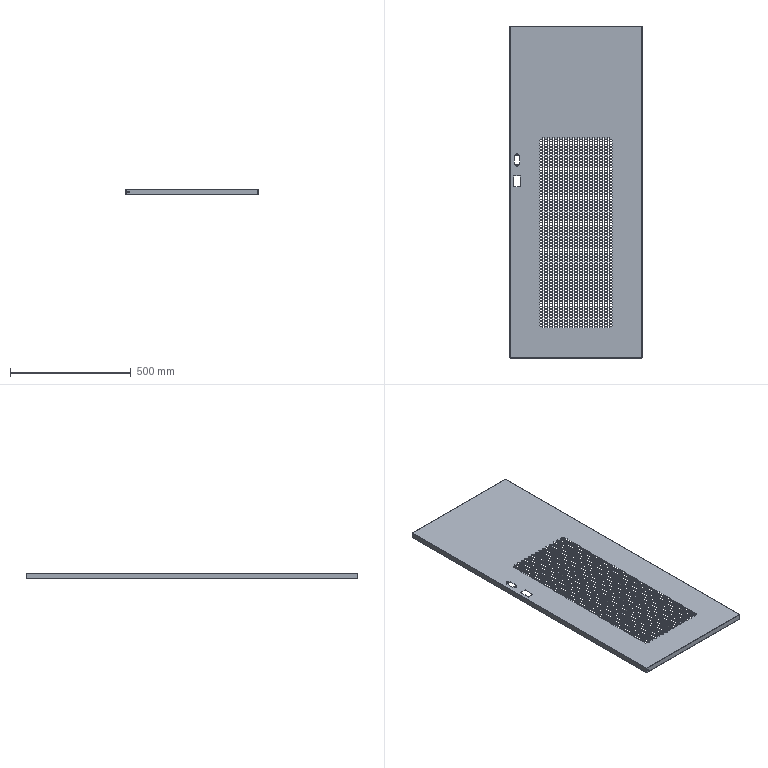Part | SolidWorks | features APattern 1, ICE 1, SplitBody 1 | 1 solid | 11528 faces | volume 901545 mm3 | plane 11452 | cylinder 60 | spline 16 | commonest cylinder face diameters 5.5 x12 6.5 x12 11.5 x12 0.2 x8 2.6 x8 4.5 x4